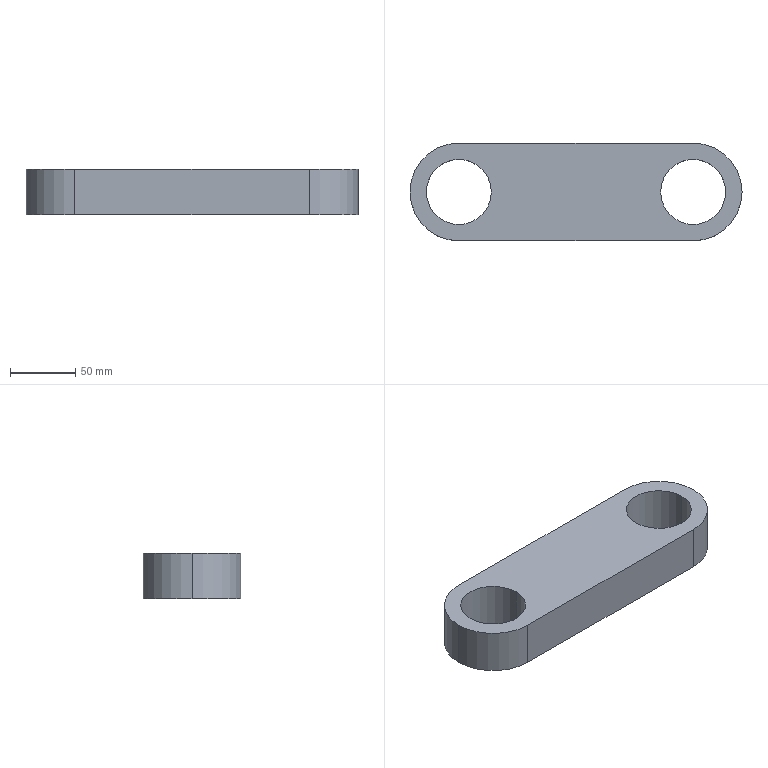Part | STEP file | LM-05-1225_default | 1 solid | 11 faces | box 255 x 75 x 35 mm | volume 489681 mm3 | cylinder 7 | plane 4 | commonest cylinder face diameters 50 x4 75 x3
STEP:
#1=CARTESIAN_POINT('',(0.,0.,0.));
#2=DIRECTION('',(0.,0.,1.));
#3=DIRECTION('',(1.,0.,0.));
#4=AXIS2_PLACEMENT_3D('',#1,#2,#3);
#5=CARTESIAN_POINT('',(65.,0.,17.5));
#6=VERTEX_POINT('',#5);
#7=CARTESIAN_POINT('',(65.,0.,-17.5));
#8=VERTEX_POINT('',#7);
#9=CARTESIAN_POINT('',(65.,0.,17.5));
#10=DIRECTION('',(0.,0.,-1.));
#11=VECTOR('',#10,1.);
#12=LINE('',#9,#11);
#13=CARTESIAN_POINT('',(90.,0.,17.5));
#14=DIRECTION('',(0.,0.,-1.));
#15=DIRECTION('',(-1.,0.,0.));
#16=AXIS2_PLACEMENT_3D('',#13,#14,#15);
#17=CYLINDRICAL_SURFACE('',#16,25.);
#18=CARTESIAN_POINT('',(6.283,0.));
#19=DIRECTION('',(0.,1.));
#20=VECTOR('',#19,1.);
#21=LINE('',#18,#20);
#22=(GEOMETRIC_REPRESENTATION_CONTEXT(2)PARAMETRIC_REPRESENTATION_CONTEXT()REPRESENTATION_CONTEXT('',''));
#23=DEFINITIONAL_REPRESENTATION('',(#21),#22);
#24=PCURVE('',#17,#23);
#25=CARTESIAN_POINT('',(90.,0.,17.5));
#26=DIRECTION('',(0.,0.,-1.));
#27=DIRECTION('',(-1.,0.,0.));
#28=AXIS2_PLACEMENT_3D('',#25,#26,#27);
#29=CYLINDRICAL_SURFACE('',#28,25.);
#30=CARTESIAN_POINT('',(0.,0.));
#31=DIRECTION('',(0.,1.));
#32=VECTOR('',#31,1.);
#33=LINE('',#30,#32);
#34=(GEOMETRIC_REPRESENTATION_CONTEXT(2)PARAMETRIC_REPRESENTATION_CONTEXT()REPRESENTATION_CONTEXT('',''));
#35=DEFINITIONAL_REPRESENTATION('',(#33),#34);
#36=PCURVE('',#29,#35);
#37=SURFACE_CURVE('',#12,(#24,#36),.PCURVE_S1.);
#38=EDGE_CURVE('',#6,#8,#37,.T.);
#39=ORIENTED_EDGE('',*,*,#38,.T.);
#40=CARTESIAN_POINT('',(115.,0.,-17.5));
#41=VERTEX_POINT('',#40);
#42=CARTESIAN_POINT('',(90.,0.,-17.5));
#43=DIRECTION('',(0.,0.,1.));
#44=DIRECTION('',(1.,0.,0.));
#45=AXIS2_PLACEMENT_3D('',#42,#43,#44);
#46=CIRCLE('',#45,25.);
#47=CARTESIAN_POINT('',(9.425,35.));
#48=DIRECTION('',(-1.,0.));
#49=VECTOR('',#48,1.);
#50=LINE('',#47,#49);
#51=(GEOMETRIC_REPRESENTATION_CONTEXT(2)PARAMETRIC_REPRESENTATION_CONTEXT()REPRESENTATION_CONTEXT('',''));
#52=DEFINITIONAL_REPRESENTATION('',(#50),#51);
#53=PCURVE('',#17,#52);
#54=CARTESIAN_POINT('',(-90.,0.,-17.5));
#55=DIRECTION('',(0.,0.,1.));
#56=DIRECTION('',(1.,0.,0.));
#57=AXIS2_PLACEMENT_3D('',#54,#55,#56);
#58=PLANE('',#57);
#59=CARTESIAN_POINT('',(180.,0.));
#60=DIRECTION('',(1.,0.));
#61=AXIS2_PLACEMENT_2D('',#59,#60);
#62=CIRCLE('',#61,25.);
#63=(GEOMETRIC_REPRESENTATION_CONTEXT(2)PARAMETRIC_REPRESENTATION_CONTEXT()REPRESENTATION_CONTEXT('',''));
#64=DEFINITIONAL_REPRESENTATION('',(#62),#63);
#65=PCURVE('',#58,#64);
#66=SURFACE_CURVE('',#46,(#53,#65),.PCURVE_S1.);
#67=EDGE_CURVE('',#8,#41,#66,.T.);
#68=ORIENTED_EDGE('',*,*,#67,.T.);
#69=CARTESIAN_POINT('',(115.,0.,17.5));
#70=VERTEX_POINT('',#69);
#71=CARTESIAN_POINT('',(115.,0.,17.5));
#72=DIRECTION('',(0.,0.,-1.));
#73=VECTOR('',#72,1.);
#74=LINE('',#71,#73);
#75=CARTESIAN_POINT('',(3.142,0.));
#76=DIRECTION('',(0.,1.));
#77=VECTOR('',#76,1.);
#78=LINE('',#75,#77);
#79=(GEOMETRIC_REPRESENTATION_CONTEXT(2)PARAMETRIC_REPRESENTATION_CONTEXT()REPRESENTATION_CONTEXT('',''));
#80=DEFINITIONAL_REPRESENTATION('',(#78),#79);
#81=PCURVE('',#17,#80);
#82=CARTESIAN_POINT('',(3.142,0.));
#83=DIRECTION('',(0.,1.));
#84=VECTOR('',#83,1.);
#85=LINE('',#82,#84);
#86=(GEOMETRIC_REPRESENTATION_CONTEXT(2)PARAMETRIC_REPRESENTATION_CONTEXT()REPRESENTATION_CONTEXT('',''));
#87=DEFINITIONAL_REPRESENTATION('',(#85),#86);
#88=PCURVE('',#29,#87);
#89=SURFACE_CURVE('',#74,(#81,#88),.PCURVE_S1.);
#90=EDGE_CURVE('',#70,#41,#89,.T.);
#91=ORIENTED_EDGE('',*,*,#90,.F.);
#92=CARTESIAN_POINT('',(90.,0.,17.5));
#93=DIRECTION('',(0.,0.,1.));
#94=DIRECTION('',(1.,0.,0.));
#95=AXIS2_PLACEMENT_3D('',#92,#93,#94);
#96=CIRCLE('',#95,25.);
#97=CARTESIAN_POINT('',(9.425,0.));
#98=DIRECTION('',(-1.,0.));
#99=VECTOR('',#98,1.);
#100=LINE('',#97,#99);
#101=(GEOMETRIC_REPRESENTATION_CONTEXT(2)PARAMETRIC_REPRESENTATION_CONTEXT()REPRESENTATION_CONTEXT('',''));
#102=DEFINITIONAL_REPRESENTATION('',(#100),#101);
#103=PCURVE('',#17,#102);
#104=CARTESIAN_POINT('',(-90.,0.,17.5));
#105=DIRECTION('',(0.,0.,1.));
#106=DIRECTION('',(1.,0.,0.));
#107=AXIS2_PLACEMENT_3D('',#104,#105,#106);
#108=PLANE('',#107);
#109=CARTESIAN_POINT('',(180.,0.));
#110=DIRECTION('',(1.,0.));
#111=AXIS2_PLACEMENT_2D('',#109,#110);
#112=CIRCLE('',#111,25.);
#113=(GEOMETRIC_REPRESENTATION_CONTEXT(2)PARAMETRIC_REPRESENTATION_CONTEXT()REPRESENTATION_CONTEXT('',''));
#114=DEFINITIONAL_REPRESENTATION('',(#112),#113);
#115=PCURVE('',#108,#114);
#116=SURFACE_CURVE('',#96,(#103,#115),.PCURVE_S1.);
#117=EDGE_CURVE('',#6,#70,#116,.T.);
#118=ORIENTED_EDGE('',*,*,#117,.F.);
#119=EDGE_LOOP('',(#39,#68,#91,#118));
#120=FACE_BOUND('',#119,.F.);
#121=ADVANCED_FACE('',(#120),#17,.F.);
#122=CARTESIAN_POINT('',(-115.,0.,17.5));
#123=VERTEX_POINT('',#122);
#124=CARTESIAN_POINT('',(-115.,0.,-17.5));
#125=VERTEX_POINT('',#124);
#126=CARTESIAN_POINT('',(-115.,0.,17.5));
#127=DIRECTION('',(0.,0.,-1.));
#128=VECTOR('',#127,1.);
#129=LINE('',#126,#128);
#130=CARTESIAN_POINT('',(-90.,0.,17.5));
#131=DIRECTION('',(0.,0.,-1.));
#132=DIRECTION('',(-1.,0.,0.));
#133=AXIS2_PLACEMENT_3D('',#130,#131,#132);
#134=CYLINDRICAL_SURFACE('',#133,25.);
#135=CARTESIAN_POINT('',(6.283,0.));
#136=DIRECTION('',(0.,1.));
#137=VECTOR('',#136,1.);
#138=LINE('',#135,#137);
#139=(GEOMETRIC_REPRESENTATION_CONTEXT(2)PARAMETRIC_REPRESENTATION_CONTEXT()REPRESENTATION_CONTEXT('',''));
#140=DEFINITIONAL_REPRESENTATION('',(#138),#139);
#141=PCURVE('',#134,#140);
#142=CARTESIAN_POINT('',(-90.,0.,17.5));
#143=DIRECTION('',(0.,0.,-1.));
#144=DIRECTION('',(-1.,0.,0.));
#145=AXIS2_PLACEMENT_3D('',#142,#143,#144);
#146=CYLINDRICAL_SURFACE('',#145,25.);
#147=CARTESIAN_POINT('',(0.,0.));
#148=DIRECTION('',(0.,1.));
#149=VECTOR('',#148,1.);
#150=LINE('',#147,#149);
#151=(GEOMETRIC_REPRESENTATION_CONTEXT(2)PARAMETRIC_REPRESENTATION_CONTEXT()REPRESENTATION_CONTEXT('',''));
#152=DEFINITIONAL_REPRESENTATION('',(#150),#151);
#153=PCURVE('',#146,#152);
#154=SURFACE_CURVE('',#129,(#141,#153),.PCURVE_S1.);
#155=EDGE_CURVE('',#123,#125,#154,.T.);
#156=ORIENTED_EDGE('',*,*,#155,.T.);
#157=CARTESIAN_POINT('',(-65.,0.,-17.5));
#158=VERTEX_POINT('',#157);
#159=CARTESIAN_POINT('',(-90.,0.,-17.5));
#160=DIRECTION('',(0.,0.,1.));
#161=DIRECTION('',(1.,0.,0.));
#162=AXIS2_PLACEMENT_3D('',#159,#160,#161);
#163=CIRCLE('',#162,25.);
#164=CARTESIAN_POINT('',(9.425,35.));
#165=DIRECTION('',(-1.,0.));
#166=VECTOR('',#165,1.);
#167=LINE('',#164,#166);
#168=(GEOMETRIC_REPRESENTATION_CONTEXT(2)PARAMETRIC_REPRESENTATION_CONTEXT()REPRESENTATION_CONTEXT('',''));
#169=DEFINITIONAL_REPRESENTATION('',(#167),#168);
#170=PCURVE('',#134,#169);
#171=CARTESIAN_POINT('',(0.,0.));
#172=DIRECTION('',(1.,0.));
#173=AXIS2_PLACEMENT_2D('',#171,#172);
#174=CIRCLE('',#173,25.);
#175=(GEOMETRIC_REPRESENTATION_CONTEXT(2)PARAMETRIC_REPRESENTATION_CONTEXT()REPRESENTATION_CONTEXT('',''));
#176=DEFINITIONAL_REPRESENTATION('',(#174),#175);
#177=PCURVE('',#58,#176);
#178=SURFACE_CURVE('',#163,(#170,#177),.PCURVE_S1.);
#179=EDGE_CURVE('',#125,#158,#178,.T.);
#180=ORIENTED_EDGE('',*,*,#179,.T.);
#181=CARTESIAN_POINT('',(-65.,0.,17.5));
#182=VERTEX_POINT('',#181);
#183=CARTESIAN_POINT('',(-65.,0.,17.5));
#184=DIRECTION('',(0.,0.,-1.));
#185=VECTOR('',#184,1.);
#186=LINE('',#183,#185);
#187=CARTESIAN_POINT('',(3.142,0.));
#188=DIRECTION('',(0.,1.));
#189=VECTOR('',#188,1.);
#190=LINE('',#187,#189);
#191=(GEOMETRIC_REPRESENTATION_CONTEXT(2)PARAMETRIC_REPRESENTATION_CONTEXT()REPRESENTATION_CONTEXT('',''));
#192=DEFINITIONAL_REPRESENTATION('',(#190),#191);
#193=PCURVE('',#134,#192);
#194=CARTESIAN_POINT('',(3.142,0.));
#195=DIRECTION('',(0.,1.));
#196=VECTOR('',#195,1.);
#197=LINE('',#194,#196);
#198=(GEOMETRIC_REPRESENTATION_CONTEXT(2)PARAMETRIC_REPRESENTATION_CONTEXT()REPRESENTATION_CONTEXT('',''));
#199=DEFINITIONAL_REPRESENTATION('',(#197),#198);
#200=PCURVE('',#146,#199);
#201=SURFACE_CURVE('',#186,(#193,#200),.PCURVE_S1.);
#202=EDGE_CURVE('',#182,#158,#201,.T.);
#203=ORIENTED_EDGE('',*,*,#202,.F.);
#204=CARTESIAN_POINT('',(-90.,0.,17.5));
#205=DIRECTION('',(0.,0.,1.));
#206=DIRECTION('',(1.,0.,0.));
#207=AXIS2_PLACEMENT_3D('',#204,#205,#206);
#208=CIRCLE('',#207,25.);
#209=CARTESIAN_POINT('',(9.425,0.));
#210=DIRECTION('',(-1.,0.));
#211=VECTOR('',#210,1.);
#212=LINE('',#209,#211);
#213=(GEOMETRIC_REPRESENTATION_CONTEXT(2)PARAMETRIC_REPRESENTATION_CONTEXT()REPRESENTATION_CONTEXT('',''));
#214=DEFINITIONAL_REPRESENTATION('',(#212),#213);
#215=PCURVE('',#134,#214);
#216=CARTESIAN_POINT('',(0.,0.));
#217=DIRECTION('',(1.,0.));
#218=AXIS2_PLACEMENT_2D('',#216,#217);
#219=CIRCLE('',#218,25.);
#220=(GEOMETRIC_REPRESENTATION_CONTEXT(2)PARAMETRIC_REPRESENTATION_CONTEXT()REPRESENTATION_CONTEXT('',''));
#221=DEFINITIONAL_REPRESENTATION('',(#219),#220);
#222=PCURVE('',#108,#221);
#223=SURFACE_CURVE('',#208,(#215,#222),.PCURVE_S1.);
#224=EDGE_CURVE('',#123,#182,#223,.T.);
#225=ORIENTED_EDGE('',*,*,#224,.F.);
#226=EDGE_LOOP('',(#156,#180,#203,#225));
#227=FACE_BOUND('',#226,.F.);
#228=ADVANCED_FACE('',(#227),#134,.F.);
#229=CARTESIAN_POINT('',(-127.5,0.,17.5));
#230=VERTEX_POINT('',#229);
#231=CARTESIAN_POINT('',(-90.,-37.5,17.5));
#232=VERTEX_POINT('',#231);
#233=CARTESIAN_POINT('',(-90.,0.,17.5));
#234=DIRECTION('',(0.,0.,1.));
#235=DIRECTION('',(1.,0.,0.));
#236=AXIS2_PLACEMENT_3D('',#233,#234,#235);
#237=CIRCLE('',#236,37.5);
#238=CARTESIAN_POINT('',(-90.,0.,17.5));
#239=DIRECTION('',(0.,0.,-1.));
#240=DIRECTION('',(-1.,0.,0.));
#241=AXIS2_PLACEMENT_3D('',#238,#239,#240);
#242=CYLINDRICAL_SURFACE('',#241,37.5);
#243=CARTESIAN_POINT('',(9.425,0.));
#244=DIRECTION('',(-1.,0.));
#245=VECTOR('',#244,1.);
#246=LINE('',#243,#245);
#247=(GEOMETRIC_REPRESENTATION_CONTEXT(2)PARAMETRIC_REPRESENTATION_CONTEXT()REPRESENTATION_CONTEXT('',''));
#248=DEFINITIONAL_REPRESENTATION('',(#246),#247);
#249=PCURVE('',#242,#248);
#250=CARTESIAN_POINT('',(0.,0.));
#251=DIRECTION('',(1.,0.));
#252=AXIS2_PLACEMENT_2D('',#250,#251);
#253=CIRCLE('',#252,37.5);
#254=(GEOMETRIC_REPRESENTATION_CONTEXT(2)PARAMETRIC_REPRESENTATION_CONTEXT()REPRESENTATION_CONTEXT('',''));
#255=DEFINITIONAL_REPRESENTATION('',(#253),#254);
#256=PCURVE('',#108,#255);
#257=SURFACE_CURVE('',#237,(#249,#256),.PCURVE_S1.);
#258=EDGE_CURVE('',#230,#232,#257,.T.);
#259=ORIENTED_EDGE('',*,*,#258,.F.);
#260=CARTESIAN_POINT('',(-127.5,0.,-17.5));
#261=VERTEX_POINT('',#260);
#262=CARTESIAN_POINT('',(-127.5,0.,17.5));
#263=DIRECTION('',(0.,0.,-1.));
#264=VECTOR('',#263,1.);
#265=LINE('',#262,#264);
#266=CARTESIAN_POINT('',(6.283,0.));
#267=DIRECTION('',(0.,1.));
#268=VECTOR('',#267,1.);
#269=LINE('',#266,#268);
#270=(GEOMETRIC_REPRESENTATION_CONTEXT(2)PARAMETRIC_REPRESENTATION_CONTEXT()REPRESENTATION_CONTEXT('',''));
#271=DEFINITIONAL_REPRESENTATION('',(#269),#270);
#272=PCURVE('',#242,#271);
#273=CARTESIAN_POINT('',(-90.,0.,17.5));
#274=DIRECTION('',(0.,0.,-1.));
#275=DIRECTION('',(-1.,0.,0.));
#276=AXIS2_PLACEMENT_3D('',#273,#274,#275);
#277=CYLINDRICAL_SURFACE('',#276,37.5);
#278=CARTESIAN_POINT('',(0.,0.));
#279=DIRECTION('',(0.,1.));
#280=VECTOR('',#279,1.);
#281=LINE('',#278,#280);
#282=(GEOMETRIC_REPRESENTATION_CONTEXT(2)PARAMETRIC_REPRESENTATION_CONTEXT()REPRESENTATION_CONTEXT('',''));
#283=DEFINITIONAL_REPRESENTATION('',(#281),#282);
#284=PCURVE('',#277,#283);
#285=SURFACE_CURVE('',#265,(#272,#284),.PCURVE_S1.);
#286=EDGE_CURVE('',#230,#261,#285,.T.);
#287=ORIENTED_EDGE('',*,*,#286,.T.);
#288=CARTESIAN_POINT('',(-90.,-37.5,-17.5));
#289=VERTEX_POINT('',#288);
#290=CARTESIAN_POINT('',(-90.,0.,-17.5));
#291=DIRECTION('',(0.,0.,1.));
#292=DIRECTION('',(1.,0.,0.));
#293=AXIS2_PLACEMENT_3D('',#290,#291,#292);
#294=CIRCLE('',#293,37.5);
#295=CARTESIAN_POINT('',(9.425,35.));
#296=DIRECTION('',(-1.,0.));
#297=VECTOR('',#296,1.);
#298=LINE('',#295,#297);
#299=(GEOMETRIC_REPRESENTATION_CONTEXT(2)PARAMETRIC_REPRESENTATION_CONTEXT()REPRESENTATION_CONTEXT('',''));
#300=DEFINITIONAL_REPRESENTATION('',(#298),#299);
#301=PCURVE('',#242,#300);
#302=CARTESIAN_POINT('',(0.,0.));
#303=DIRECTION('',(1.,0.));
#304=AXIS2_PLACEMENT_2D('',#302,#303);
#305=CIRCLE('',#304,37.5);
#306=(GEOMETRIC_REPRESENTATION_CONTEXT(2)PARAMETRIC_REPRESENTATION_CONTEXT()REPRESENTATION_CONTEXT('',''));
#307=DEFINITIONAL_REPRESENTATION('',(#305),#306);
#308=PCURVE('',#58,#307);
#309=SURFACE_CURVE('',#294,(#301,#308),.PCURVE_S1.);
#310=EDGE_CURVE('',#261,#289,#309,.T.);
#311=ORIENTED_EDGE('',*,*,#310,.T.);
#312=CARTESIAN_POINT('',(-90.,-37.5,17.5));
#313=DIRECTION('',(0.,0.,-1.));
#314=VECTOR('',#313,1.);
#315=LINE('',#312,#314);
#316=CARTESIAN_POINT('',(4.712,0.));
#317=DIRECTION('',(0.,1.));
#318=VECTOR('',#317,1.);
#319=LINE('',#316,#318);
#320=(GEOMETRIC_REPRESENTATION_CONTEXT(2)PARAMETRIC_REPRESENTATION_CONTEXT()REPRESENTATION_CONTEXT('',''));
#321=DEFINITIONAL_REPRESENTATION('',(#319),#320);
#322=PCURVE('',#242,#321);
#323=CARTESIAN_POINT('',(-90.,-37.5,17.5));
#324=DIRECTION('',(0.,1.,0.));
#325=DIRECTION('',(-1.,0.,0.));
#326=AXIS2_PLACEMENT_3D('',#323,#324,#325);
#327=PLANE('',#326);
#328=CARTESIAN_POINT('',(0.,0.));
#329=DIRECTION('',(0.,-1.));
#330=VECTOR('',#329,1.);
#331=LINE('',#328,#330);
#332=(GEOMETRIC_REPRESENTATION_CONTEXT(2)PARAMETRIC_REPRESENTATION_CONTEXT()REPRESENTATION_CONTEXT('',''));
#333=DEFINITIONAL_REPRESENTATION('',(#331),#332);
#334=PCURVE('',#327,#333);
#335=SURFACE_CURVE('',#315,(#322,#334),.PCURVE_S1.);
#336=EDGE_CURVE('',#232,#289,#335,.T.);
#337=ORIENTED_EDGE('',*,*,#336,.F.);
#338=EDGE_LOOP('',(#259,#287,#311,#337));
#339=FACE_BOUND('',#338,.T.);
#340=ADVANCED_FACE('',(#339),#242,.T.);
#341=ORIENTED_EDGE('',*,*,#224,.F.);
#342=CARTESIAN_POINT('',(-90.,0.,17.5));
#343=DIRECTION('',(0.,0.,1.));
#344=DIRECTION('',(1.,0.,0.));
#345=AXIS2_PLACEMENT_3D('',#342,#343,#344);
#346=CIRCLE('',#345,25.);
#347=CARTESIAN_POINT('',(0.,0.));
#348=DIRECTION('',(1.,0.));
#349=AXIS2_PLACEMENT_2D('',#347,#348);
#350=CIRCLE('',#349,25.);
#351=(GEOMETRIC_REPRESENTATION_CONTEXT(2)PARAMETRIC_REPRESENTATION_CONTEXT()REPRESENTATION_CONTEXT('',''));
#352=DEFINITIONAL_REPRESENTATION('',(#350),#351);
#353=PCURVE('',#108,#352);
#354=CARTESIAN_POINT('',(3.142,0.));
#355=DIRECTION('',(-1.,0.));
#356=VECTOR('',#355,1.);
#357=LINE('',#354,#356);
#358=(GEOMETRIC_REPRESENTATION_CONTEXT(2)PARAMETRIC_REPRESENTATION_CONTEXT()REPRESENTATION_CONTEXT('',''));
#359=DEFINITIONAL_REPRESENTATION('',(#357),#358);
#360=PCURVE('',#146,#359);
#361=SURFACE_CURVE('',#346,(#353,#360),.PCURVE_S1.);
#362=EDGE_CURVE('',#182,#123,#361,.T.);
#363=ORIENTED_EDGE('',*,*,#362,.F.);
#364=EDGE_LOOP('',(#341,#363));
#365=FACE_BOUND('',#364,.T.);
#366=CARTESIAN_POINT('',(-90.,37.5,17.5));
#367=VERTEX_POINT('',#366);
#368=CARTESIAN_POINT('',(-90.,0.,17.5));
#369=DIRECTION('',(0.,0.,1.));
#370=DIRECTION('',(1.,0.,0.));
#371=AXIS2_PLACEMENT_3D('',#368,#369,#370);
#372=CIRCLE('',#371,37.5);
#373=CARTESIAN_POINT('',(0.,0.));
#374=DIRECTION('',(1.,0.));
#375=AXIS2_PLACEMENT_2D('',#373,#374);
#376=CIRCLE('',#375,37.5);
#377=(GEOMETRIC_REPRESENTATION_CONTEXT(2)PARAMETRIC_REPRESENTATION_CONTEXT()REPRESENTATION_CONTEXT('',''));
#378=DEFINITIONAL_REPRESENTATION('',(#376),#377);
#379=PCURVE('',#108,#378);
#380=CARTESIAN_POINT('',(3.142,0.));
#381=DIRECTION('',(-1.,0.));
#382=VECTOR('',#381,1.);
#383=LINE('',#380,#382);
#384=(GEOMETRIC_REPRESENTATION_CONTEXT(2)PARAMETRIC_REPRESENTATION_CONTEXT()REPRESENTATION_CONTEXT('',''));
#385=DEFINITIONAL_REPRESENTATION('',(#383),#384);
#386=PCURVE('',#277,#385);
#387=SURFACE_CURVE('',#372,(#379,#386),.PCURVE_S1.);
#388=EDGE_CURVE('',#367,#230,#387,.T.);
#389=ORIENTED_EDGE('',*,*,#388,.T.);
#390=ORIENTED_EDGE('',*,*,#258,.T.);
#391=CARTESIAN_POINT('',(90.,-37.5,17.5));
#392=VERTEX_POINT('',#391);
#393=CARTESIAN_POINT('',(-90.,-37.5,17.5));
#394=DIRECTION('',(1.,0.,0.));
#395=VECTOR('',#394,1.);
#396=LINE('',#393,#395);
#397=CARTESIAN_POINT('',(0.,-37.5));
#398=DIRECTION('',(1.,0.));
#399=VECTOR('',#398,1.);
#400=LINE('',#397,#399);
#401=(GEOMETRIC_REPRESENTATION_CONTEXT(2)PARAMETRIC_REPRESENTATION_CONTEXT()REPRESENTATION_CONTEXT('',''));
#402=DEFINITIONAL_REPRESENTATION('',(#400),#401);
#403=PCURVE('',#108,#402);
#404=CARTESIAN_POINT('',(0.,0.));
#405=DIRECTION('',(-1.,0.));
#406=VECTOR('',#405,1.);
#407=LINE('',#404,#406);
#408=(GEOMETRIC_REPRESENTATION_CONTEXT(2)PARAMETRIC_REPRESENTATION_CONTEXT()REPRESENTATION_CONTEXT('',''));
#409=DEFINITIONAL_REPRESENTATION('',(#407),#408);
#410=PCURVE('',#327,#409);
#411=SURFACE_CURVE('',#396,(#403,#410),.PCURVE_S1.);
#412=EDGE_CURVE('',#232,#392,#411,.T.);
#413=ORIENTED_EDGE('',*,*,#412,.T.);
#414=CARTESIAN_POINT('',(90.,37.5,17.5));
#415=VERTEX_POINT('',#414);
#416=CARTESIAN_POINT('',(90.,0.,17.5));
#417=DIRECTION('',(0.,0.,1.));
#418=DIRECTION('',(1.,0.,0.));
#419=AXIS2_PLACEMENT_3D('',#416,#417,#418);
#420=CIRCLE('',#419,37.5);
#421=CARTESIAN_POINT('',(180.,0.));
#422=DIRECTION('',(1.,0.));
#423=AXIS2_PLACEMENT_2D('',#421,#422);
#424=CIRCLE('',#423,37.5);
#425=(GEOMETRIC_REPRESENTATION_CONTEXT(2)PARAMETRIC_REPRESENTATION_CONTEXT()REPRESENTATION_CONTEXT('',''));
#426=DEFINITIONAL_REPRESENTATION('',(#424),#425);
#427=PCURVE('',#108,#426);
#428=CARTESIAN_POINT('',(90.,0.,17.5));
#429=DIRECTION('',(0.,0.,-1.));
#430=DIRECTION('',(-1.,0.,0.));
#431=AXIS2_PLACEMENT_3D('',#428,#429,#430);
#432=CYLINDRICAL_SURFACE('',#431,37.5);
#433=CARTESIAN_POINT('',(9.425,0.));
#434=DIRECTION('',(-1.,0.));
#435=VECTOR('',#434,1.);
#436=LINE('',#433,#435);
#437=(GEOMETRIC_REPRESENTATION_CONTEXT(2)PARAMETRIC_REPRESENTATION_CONTEXT()REPRESENTATION_CONTEXT('',''));
#438=DEFINITIONAL_REPRESENTATION('',(#436),#437);
#439=PCURVE('',#432,#438);
#440=SURFACE_CURVE('',#420,(#427,#439),.PCURVE_S1.);
#441=EDGE_CURVE('',#392,#415,#440,.T.);
#442=ORIENTED_EDGE('',*,*,#441,.T.);
#443=CARTESIAN_POINT('',(-90.,37.5,17.5));
#444=DIRECTION('',(-1.,0.,0.));
#445=VECTOR('',#444,1.);
#446=LINE('',#443,#445);
#447=CARTESIAN_POINT('',(0.,37.5));
#448=DIRECTION('',(-1.,0.));
#449=VECTOR('',#448,1.);
#450=LINE('',#447,#449);
#451=(GEOMETRIC_REPRESENTATION_CONTEXT(2)PARAMETRIC_REPRESENTATION_CONTEXT()REPRESENTATION_CONTEXT('',''));
#452=DEFINITIONAL_REPRESENTATION('',(#450),#451);
#453=PCURVE('',#108,#452);
#454=CARTESIAN_POINT('',(-90.,37.5,17.5));
#455=DIRECTION('',(0.,-1.,0.));
#456=DIRECTION('',(1.,0.,0.));
#457=AXIS2_PLACEMENT_3D('',#454,#455,#456);
#458=PLANE('',#457);
#459=CARTESIAN_POINT('',(0.,0.));
#460=DIRECTION('',(-1.,0.));
#461=VECTOR('',#460,1.);
#462=LINE('',#459,#461);
#463=(GEOMETRIC_REPRESENTATION_CONTEXT(2)PARAMETRIC_REPRESENTATION_CONTEXT()REPRESENTATION_CONTEXT('',''));
#464=DEFINITIONAL_REPRESENTATION('',(#462),#463);
#465=PCURVE('',#458,#464);
#466=SURFACE_CURVE('',#446,(#453,#465),.PCURVE_S1.);
#467=EDGE_CURVE('',#415,#367,#466,.T.);
#468=ORIENTED_EDGE('',*,*,#467,.T.);
#469=EDGE_LOOP('',(#389,#390,#413,#442,#468));
#470=FACE_BOUND('',#469,.T.);
#471=ORIENTED_EDGE('',*,*,#117,.F.);
#472=CARTESIAN_POINT('',(90.,0.,17.5));
#473=DIRECTION('',(0.,0.,1.));
#474=DIRECTION('',(1.,0.,0.));
#475=AXIS2_PLACEMENT_3D('',#472,#473,#474);
#476=CIRCLE('',#475,25.);
#477=CARTESIAN_POINT('',(180.,0.));
#478=DIRECTION('',(1.,0.));
#479=AXIS2_PLACEMENT_2D('',#477,#478);
#480=CIRCLE('',#479,25.);
#481=(GEOMETRIC_REPRESENTATION_CONTEXT(2)PARAMETRIC_REPRESENTATION_CONTEXT()REPRESENTATION_CONTEXT('',''));
#482=DEFINITIONAL_REPRESENTATION('',(#480),#481);
#483=PCURVE('',#108,#482);
#484=CARTESIAN_POINT('',(3.142,0.));
#485=DIRECTION('',(-1.,0.));
#486=VECTOR('',#485,1.);
#487=LINE('',#484,#486);
#488=(GEOMETRIC_REPRESENTATION_CONTEXT(2)PARAMETRIC_REPRESENTATION_CONTEXT()REPRESENTATION_CONTEXT('',''));
#489=DEFINITIONAL_REPRESENTATION('',(#487),#488);
#490=PCURVE('',#29,#489);
#491=SURFACE_CURVE('',#476,(#483,#490),.PCURVE_S1.);
#492=EDGE_CURVE('',#70,#6,#491,.T.);
#493=ORIENTED_EDGE('',*,*,#492,.F.);
#494=EDGE_LOOP('',(#471,#493));
#495=FACE_BOUND('',#494,.T.);
#496=ADVANCED_FACE('',(#365,#470,#495),#108,.T.);
#497=CARTESIAN_POINT('',(-90.,37.5,-17.5));
#498=VERTEX_POINT('',#497);
#499=CARTESIAN_POINT('',(-90.,0.,-17.5));
#500=DIRECTION('',(0.,0.,1.));
#501=DIRECTION('',(1.,0.,0.));
#502=AXIS2_PLACEMENT_3D('',#499,#500,#501);
#503=CIRCLE('',#502,37.5);
#504=CARTESIAN_POINT('',(0.,0.));
#505=DIRECTION('',(1.,0.));
#506=AXIS2_PLACEMENT_2D('',#504,#505);
#507=CIRCLE('',#506,37.5);
#508=(GEOMETRIC_REPRESENTATION_CONTEXT(2)PARAMETRIC_REPRESENTATION_CONTEXT()REPRESENTATION_CONTEXT('',''));
#509=DEFINITIONAL_REPRESENTATION('',(#507),#508);
#510=PCURVE('',#58,#509);
#511=CARTESIAN_POINT('',(3.142,35.));
#512=DIRECTION('',(-1.,0.));
#513=VECTOR('',#512,1.);
#514=LINE('',#511,#513);
#515=(GEOMETRIC_REPRESENTATION_CONTEXT(2)PARAMETRIC_REPRESENTATION_CONTEXT()REPRESENTATION_CONTEXT('',''));
#516=DEFINITIONAL_REPRESENTATION('',(#514),#515);
#517=PCURVE('',#277,#516);
#518=SURFACE_CURVE('',#503,(#510,#517),.PCURVE_S1.);
#519=EDGE_CURVE('',#498,#261,#518,.T.);
#520=ORIENTED_EDGE('',*,*,#519,.F.);
#521=CARTESIAN_POINT('',(90.,37.5,-17.5));
#522=VERTEX_POINT('',#521);
#523=CARTESIAN_POINT('',(-90.,37.5,-17.5));
#524=DIRECTION('',(-1.,0.,0.));
#525=VECTOR('',#524,1.);
#526=LINE('',#523,#525);
#527=CARTESIAN_POINT('',(0.,37.5));
#528=DIRECTION('',(-1.,0.));
#529=VECTOR('',#528,1.);
#530=LINE('',#527,#529);
#531=(GEOMETRIC_REPRESENTATION_CONTEXT(2)PARAMETRIC_REPRESENTATION_CONTEXT()REPRESENTATION_CONTEXT('',''));
#532=DEFINITIONAL_REPRESENTATION('',(#530),#531);
#533=PCURVE('',#58,#532);
#534=CARTESIAN_POINT('',(0.,-35.));
#535=DIRECTION('',(-1.,0.));
#536=VECTOR('',#535,1.);
#537=LINE('',#534,#536);
#538=(GEOMETRIC_REPRESENTATION_CONTEXT(2)PARAMETRIC_REPRESENTATION_CONTEXT()REPRESENTATION_CONTEXT('',''));
#539=DEFINITIONAL_REPRESENTATION('',(#537),#538);
#540=PCURVE('',#458,#539);
#541=SURFACE_CURVE('',#526,(#533,#540),.PCURVE_S1.);
#542=EDGE_CURVE('',#522,#498,#541,.T.);
#543=ORIENTED_EDGE('',*,*,#542,.F.);
#544=CARTESIAN_POINT('',(90.,-37.5,-17.5));
#545=VERTEX_POINT('',#544);
#546=CARTESIAN_POINT('',(90.,0.,-17.5));
#547=DIRECTION('',(0.,0.,1.));
#548=DIRECTION('',(1.,0.,0.));
#549=AXIS2_PLACEMENT_3D('',#546,#547,#548);
#550=CIRCLE('',#549,37.5);
#551=CARTESIAN_POINT('',(180.,0.));
#552=DIRECTION('',(1.,0.));
#553=AXIS2_PLACEMENT_2D('',#551,#552);
#554=CIRCLE('',#553,37.5);
#555=(GEOMETRIC_REPRESENTATION_CONTEXT(2)PARAMETRIC_REPRESENTATION_CONTEXT()REPRESENTATION_CONTEXT('',''));
#556=DEFINITIONAL_REPRESENTATION('',(#554),#555);
#557=PCURVE('',#58,#556);
#558=CARTESIAN_POINT('',(9.425,35.));
#559=DIRECTION('',(-1.,0.));
#560=VECTOR('',#559,1.);
#561=LINE('',#558,#560);
#562=(GEOMETRIC_REPRESENTATION_CONTEXT(2)PARAMETRIC_REPRESENTATION_CONTEXT()REPRESENTATION_CONTEXT('',''));
#563=DEFINITIONAL_REPRESENTATION('',(#561),#562);
#564=PCURVE('',#432,#563);
#565=SURFACE_CURVE('',#550,(#557,#564),.PCURVE_S1.);
#566=EDGE_CURVE('',#545,#522,#565,.T.);
#567=ORIENTED_EDGE('',*,*,#566,.F.);
#568=CARTESIAN_POINT('',(-90.,-37.5,-17.5));
#569=DIRECTION('',(1.,0.,0.));
#570=VECTOR('',#569,1.);
#571=LINE('',#568,#570);
#572=CARTESIAN_POINT('',(0.,-37.5));
#573=DIRECTION('',(1.,0.));
#574=VECTOR('',#573,1.);
#575=LINE('',#572,#574);
#576=(GEOMETRIC_REPRESENTATION_CONTEXT(2)PARAMETRIC_REPRESENTATION_CONTEXT()REPRESENTATION_CONTEXT('',''));
#577=DEFINITIONAL_REPRESENTATION('',(#575),#576);
#578=PCURVE('',#58,#577);
#579=CARTESIAN_POINT('',(0.,-35.));
#580=DIRECTION('',(-1.,0.));
#581=VECTOR('',#580,1.);
#582=LINE('',#579,#581);
#583=(GEOMETRIC_REPRESENTATION_CONTEXT(2)PARAMETRIC_REPRESENTATION_CONTEXT()REPRESENTATION_CONTEXT('',''));
#584=DEFINITIONAL_REPRESENTATION('',(#582),#583);
#585=PCURVE('',#327,#584);
#586=SURFACE_CURVE('',#571,(#578,#585),.PCURVE_S1.);
#587=EDGE_CURVE('',#289,#545,#586,.T.);
#588=ORIENTED_EDGE('',*,*,#587,.F.);
#589=ORIENTED_EDGE('',*,*,#310,.F.);
#590=EDGE_LOOP('',(#520,#543,#567,#588,#589));
#591=FACE_BOUND('',#590,.T.);
#592=ORIENTED_EDGE('',*,*,#179,.T.);
#593=CARTESIAN_POINT('',(-90.,0.,-17.5));
#594=DIRECTION('',(0.,0.,1.));
#595=DIRECTION('',(1.,0.,0.));
#596=AXIS2_PLACEMENT_3D('',#593,#594,#595);
#597=CIRCLE('',#596,25.);
#598=CARTESIAN_POINT('',(0.,0.));
#599=DIRECTION('',(1.,0.));
#600=AXIS2_PLACEMENT_2D('',#598,#599);
#601=CIRCLE('',#600,25.);
#602=(GEOMETRIC_REPRESENTATION_CONTEXT(2)PARAMETRIC_REPRESENTATION_CONTEXT()REPRESENTATION_CONTEXT('',''));
#603=DEFINITIONAL_REPRESENTATION('',(#601),#602);
#604=PCURVE('',#58,#603);
#605=CARTESIAN_POINT('',(3.142,35.));
#606=DIRECTION('',(-1.,0.));
#607=VECTOR('',#606,1.);
#608=LINE('',#605,#607);
#609=(GEOMETRIC_REPRESENTATION_CONTEXT(2)PARAMETRIC_REPRESENTATION_CONTEXT()REPRESENTATION_CONTEXT('',''));
#610=DEFINITIONAL_REPRESENTATION('',(#608),#609);
#611=PCURVE('',#146,#610);
#612=SURFACE_CURVE('',#597,(#604,#611),.PCURVE_S1.);
#613=EDGE_CURVE('',#158,#125,#612,.T.);
#614=ORIENTED_EDGE('',*,*,#613,.T.);
#615=EDGE_LOOP('',(#592,#614));
#616=FACE_BOUND('',#615,.T.);
#617=ORIENTED_EDGE('',*,*,#67,.T.);
#618=CARTESIAN_POINT('',(90.,0.,-17.5));
#619=DIRECTION('',(0.,0.,1.));
#620=DIRECTION('',(1.,0.,0.));
#621=AXIS2_PLACEMENT_3D('',#618,#619,#620);
#622=CIRCLE('',#621,25.);
#623=CARTESIAN_POINT('',(180.,0.));
#624=DIRECTION('',(1.,0.));
#625=AXIS2_PLACEMENT_2D('',#623,#624);
#626=CIRCLE('',#625,25.);
#627=(GEOMETRIC_REPRESENTATION_CONTEXT(2)PARAMETRIC_REPRESENTATION_CONTEXT()REPRESENTATION_CONTEXT('',''));
#628=DEFINITIONAL_REPRESENTATION('',(#626),#627);
#629=PCURVE('',#58,#628);
#630=CARTESIAN_POINT('',(3.142,35.));
#631=DIRECTION('',(-1.,0.));
#632=VECTOR('',#631,1.);
#633=LINE('',#630,#632);
#634=(GEOMETRIC_REPRESENTATION_CONTEXT(2)PARAMETRIC_REPRESENTATION_CONTEXT()REPRESENTATION_CONTEXT('',''));
#635=DEFINITIONAL_REPRESENTATION('',(#633),#634);
#636=PCURVE('',#29,#635);
#637=SURFACE_CURVE('',#622,(#629,#636),.PCURVE_S1.);
#638=EDGE_CURVE('',#41,#8,#637,.T.);
#639=ORIENTED_EDGE('',*,*,#638,.T.);
#640=EDGE_LOOP('',(#617,#639));
#641=FACE_BOUND('',#640,.T.);
#642=ADVANCED_FACE('',(#591,#616,#641),#58,.F.);
#643=ORIENTED_EDGE('',*,*,#286,.F.);
#644=ORIENTED_EDGE('',*,*,#388,.F.);
#645=CARTESIAN_POINT('',(-90.,37.5,17.5));
#646=DIRECTION('',(0.,0.,-1.));
#647=VECTOR('',#646,1.);
#648=LINE('',#645,#647);
#649=CARTESIAN_POINT('',(1.571,0.));
#650=DIRECTION('',(0.,1.));
#651=VECTOR('',#650,1.);
#652=LINE('',#649,#651);
#653=(GEOMETRIC_REPRESENTATION_CONTEXT(2)PARAMETRIC_REPRESENTATION_CONTEXT()REPRESENTATION_CONTEXT('',''));
#654=DEFINITIONAL_REPRESENTATION('',(#652),#653);
#655=PCURVE('',#277,#654);
#656=CARTESIAN_POINT('',(0.,0.));
#657=DIRECTION('',(0.,-1.));
#658=VECTOR('',#657,1.);
#659=LINE('',#656,#658);
#660=(GEOMETRIC_REPRESENTATION_CONTEXT(2)PARAMETRIC_REPRESENTATION_CONTEXT()REPRESENTATION_CONTEXT('',''));
#661=DEFINITIONAL_REPRESENTATION('',(#659),#660);
#662=PCURVE('',#458,#661);
#663=SURFACE_CURVE('',#648,(#655,#662),.PCURVE_S1.);
#664=EDGE_CURVE('',#367,#498,#663,.T.);
#665=ORIENTED_EDGE('',*,*,#664,.T.);
#666=ORIENTED_EDGE('',*,*,#519,.T.);
#667=EDGE_LOOP('',(#643,#644,#665,#666));
#668=FACE_BOUND('',#667,.T.);
#669=ADVANCED_FACE('',(#668),#277,.T.);
#670=ORIENTED_EDGE('',*,*,#587,.T.);
#671=CARTESIAN_POINT('',(90.,-37.5,17.5));
#672=DIRECTION('',(0.,0.,-1.));
#673=VECTOR('',#672,1.);
#674=LINE('',#671,#673);
#675=CARTESIAN_POINT('',(-180.,0.));
#676=DIRECTION('',(0.,-1.));
#677=VECTOR('',#676,1.);
#678=LINE('',#675,#677);
#679=(GEOMETRIC_REPRESENTATION_CONTEXT(2)PARAMETRIC_REPRESENTATION_CONTEXT()REPRESENTATION_CONTEXT('',''));
#680=DEFINITIONAL_REPRESENTATION('',(#678),#679);
#681=PCURVE('',#327,#680);
#682=CARTESIAN_POINT('',(4.712,0.));
#683=DIRECTION('',(0.,1.));
#684=VECTOR('',#683,1.);
#685=LINE('',#682,#684);
#686=(GEOMETRIC_REPRESENTATION_CONTEXT(2)PARAMETRIC_REPRESENTATION_CONTEXT()REPRESENTATION_CONTEXT('',''));
#687=DEFINITIONAL_REPRESENTATION('',(#685),#686);
#688=PCURVE('',#432,#687);
#689=SURFACE_CURVE('',#674,(#681,#688),.PCURVE_S1.);
#690=EDGE_CURVE('',#392,#545,#689,.T.);
#691=ORIENTED_EDGE('',*,*,#690,.F.);
#692=ORIENTED_EDGE('',*,*,#412,.F.);
#693=ORIENTED_EDGE('',*,*,#336,.T.);
#694=EDGE_LOOP('',(#670,#691,#692,#693));
#695=FACE_BOUND('',#694,.T.);
#696=ADVANCED_FACE('',(#695),#327,.F.);
#697=ORIENTED_EDGE('',*,*,#566,.T.);
#698=CARTESIAN_POINT('',(90.,37.5,17.5));
#699=DIRECTION('',(0.,0.,-1.));
#700=VECTOR('',#699,1.);
#701=LINE('',#698,#700);
#702=CARTESIAN_POINT('',(1.571,0.));
#703=DIRECTION('',(0.,1.));
#704=VECTOR('',#703,1.);
#705=LINE('',#702,#704);
#706=(GEOMETRIC_REPRESENTATION_CONTEXT(2)PARAMETRIC_REPRESENTATION_CONTEXT()REPRESENTATION_CONTEXT('',''));
#707=DEFINITIONAL_REPRESENTATION('',(#705),#706);
#708=PCURVE('',#432,#707);
#709=CARTESIAN_POINT('',(180.,0.));
#710=DIRECTION('',(0.,-1.));
#711=VECTOR('',#710,1.);
#712=LINE('',#709,#711);
#713=(GEOMETRIC_REPRESENTATION_CONTEXT(2)PARAMETRIC_REPRESENTATION_CONTEXT()REPRESENTATION_CONTEXT('',''));
#714=DEFINITIONAL_REPRESENTATION('',(#712),#713);
#715=PCURVE('',#458,#714);
#716=SURFACE_CURVE('',#701,(#708,#715),.PCURVE_S1.);
#717=EDGE_CURVE('',#415,#522,#716,.T.);
#718=ORIENTED_EDGE('',*,*,#717,.F.);
#719=ORIENTED_EDGE('',*,*,#441,.F.);
#720=ORIENTED_EDGE('',*,*,#690,.T.);
#721=EDGE_LOOP('',(#697,#718,#719,#720));
#722=FACE_BOUND('',#721,.T.);
#723=ADVANCED_FACE('',(#722),#432,.T.);
#724=ORIENTED_EDGE('',*,*,#542,.T.);
#725=ORIENTED_EDGE('',*,*,#664,.F.);
#726=ORIENTED_EDGE('',*,*,#467,.F.);
#727=ORIENTED_EDGE('',*,*,#717,.T.);
#728=EDGE_LOOP('',(#724,#725,#726,#727));
#729=FACE_BOUND('',#728,.T.);
#730=ADVANCED_FACE('',(#729),#458,.F.);
#731=ORIENTED_EDGE('',*,*,#613,.T.);
#732=ORIENTED_EDGE('',*,*,#155,.F.);
#733=ORIENTED_EDGE('',*,*,#362,.F.);
#734=ORIENTED_EDGE('',*,*,#202,.T.);
#735=EDGE_LOOP('',(#731,#732,#733,#734));
#736=FACE_BOUND('',#735,.F.);
#737=ADVANCED_FACE('',(#736),#146,.F.);
#738=ORIENTED_EDGE('',*,*,#638,.T.);
#739=ORIENTED_EDGE('',*,*,#38,.F.);
#740=ORIENTED_EDGE('',*,*,#492,.F.);
#741=ORIENTED_EDGE('',*,*,#90,.T.);
#742=EDGE_LOOP('',(#738,#739,#740,#741));
#743=FACE_BOUND('',#742,.F.);
#744=ADVANCED_FACE('',(#743),#29,.F.);
#745=CLOSED_SHELL('',(#121,#228,#340,#496,#642,#669,#696,#723,#730,#737,#744));
#746=MANIFOLD_SOLID_BREP('',#745);
#747=(LENGTH_UNIT()NAMED_UNIT(*)SI_UNIT(.MILLI.,.METRE.));
#748=UNCERTAINTY_MEASURE_WITH_UNIT(LENGTH_MEASURE(0.0000001),#747,'','');
#749=(NAMED_UNIT(*)PLANE_ANGLE_UNIT()SI_UNIT($,.RADIAN.));
#750=(NAMED_UNIT(*)SI_UNIT($,.STERADIAN.)SOLID_ANGLE_UNIT());
#751=(GEOMETRIC_REPRESENTATION_CONTEXT(3)GLOBAL_UNCERTAINTY_ASSIGNED_CONTEXT((#748))GLOBAL_UNIT_ASSIGNED_CONTEXT((#747,#749,#750))REPRESENTATION_CONTEXT('',''));
#752=ADVANCED_BREP_SHAPE_REPRESENTATION('',(#4,#746),#751);